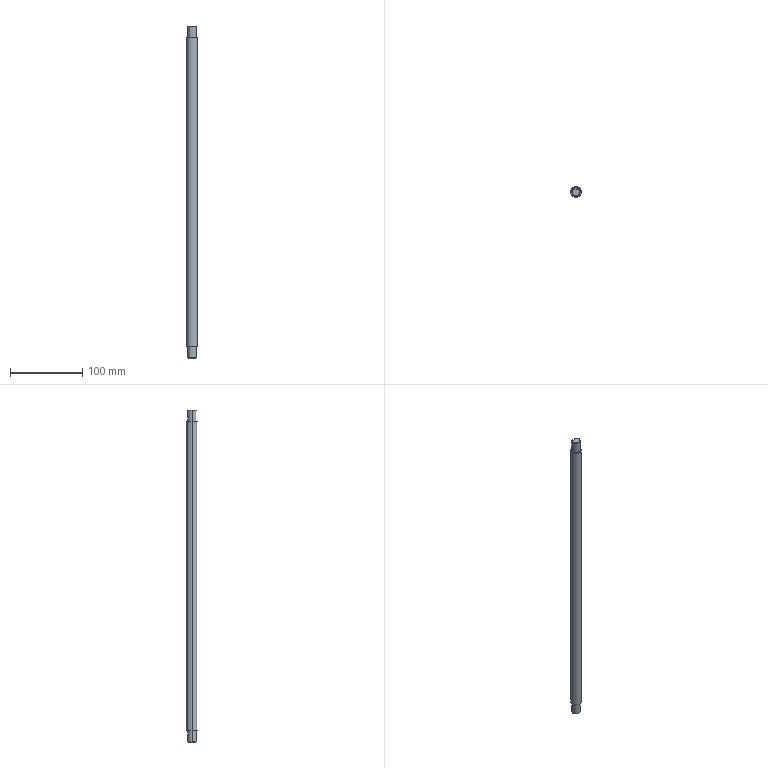Part | STEP file | 1 solid | 32 faces | box 15 x 15 x 460 mm | volume 78936 mm3 | cylinder 12 | cone 10 | plane 10 | commonest cylinder face diameters 12 x6 4 x4 15 x2